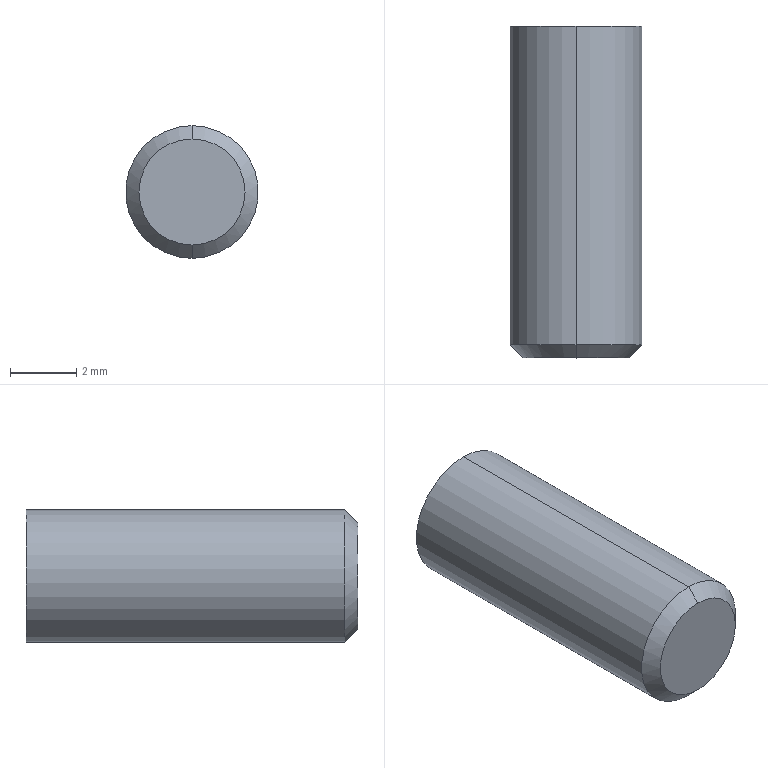Part | SolidWorks | features BaseBody 1 | 1 solid | 13 faces | box 4 x 10 x 4 mm | volume 117.243 mm3 | plane 9 | cylinder 2 | cone 2 | commonest cylinder face diameters 4 x2
STEP:
#1=CARTESIAN_POINT('',(0.,15.,10.));
#2=VERTEX_POINT('',#1);
#3=CARTESIAN_POINT('',(0.,15.,14.));
#4=VERTEX_POINT('',#3);
#5=CARTESIAN_POINT('',(0.,15.,12.));
#6=DIRECTION('',(0.,-1.,0.));
#7=DIRECTION('',(0.,0.,-1.));
#8=AXIS2_PLACEMENT_3D('',#5,#6,#7);
#9=CIRCLE('',#8,2.);
#10=EDGE_CURVE('',#2,#4,#9,.T.);
#11=ORIENTED_EDGE('',*,*,#10,.T.);
#12=CARTESIAN_POINT('',(0.,5.4,14.));
#13=VERTEX_POINT('',#12);
#14=CARTESIAN_POINT('',(0.,10.2,14.));
#15=DIRECTION('',(0.,-1.,0.));
#16=VECTOR('',#15,1000.);
#17=LINE('',#14,#16);
#18=EDGE_CURVE('',#4,#13,#17,.T.);
#19=ORIENTED_EDGE('',*,*,#18,.T.);
#20=CARTESIAN_POINT('',(0.,5.4,10.));
#21=VERTEX_POINT('',#20);
#22=CARTESIAN_POINT('',(0.,5.4,12.));
#23=DIRECTION('',(0.,1.,0.));
#24=DIRECTION('',(0.,0.,-1.));
#25=AXIS2_PLACEMENT_3D('',#22,#23,#24);
#26=CIRCLE('',#25,2.);
#27=EDGE_CURVE('',#13,#21,#26,.T.);
#28=ORIENTED_EDGE('',*,*,#27,.T.);
#29=CARTESIAN_POINT('',(0.,10.2,10.));
#30=DIRECTION('',(0.,-1.,0.));
#31=VECTOR('',#30,1000.);
#32=LINE('',#29,#31);
#33=EDGE_CURVE('',#2,#21,#32,.T.);
#34=ORIENTED_EDGE('',*,*,#33,.F.);
#35=EDGE_LOOP('',(#11,#19,#28,#34));
#36=FACE_OUTER_BOUND('',#35,.T.);
#37=CARTESIAN_POINT('',(0.,10.2,12.));
#38=DIRECTION('',(0.,-1.,0.));
#39=DIRECTION('',(0.,0.,-1.));
#40=AXIS2_PLACEMENT_3D('',#37,#38,#39);
#41=CYLINDRICAL_SURFACE('',#40,2.);
#42=ADVANCED_FACE('',(#36),#41,.T.);
#43=CARTESIAN_POINT('',(0.,5.,13.6));
#44=VERTEX_POINT('',#43);
#45=CARTESIAN_POINT('',(0.,5.,10.4));
#46=VERTEX_POINT('',#45);
#47=CARTESIAN_POINT('',(0.,5.,12.));
#48=DIRECTION('',(0.,1.,0.));
#49=DIRECTION('',(0.,0.,1.));
#50=AXIS2_PLACEMENT_3D('',#47,#48,#49);
#51=CIRCLE('',#50,1.6);
#52=EDGE_CURVE('',#44,#46,#51,.T.);
#53=ORIENTED_EDGE('',*,*,#52,.T.);
#54=CARTESIAN_POINT('',(0.,5.4,10.));
#55=DIRECTION('',(0.,0.7071,-0.7071));
#56=VECTOR('',#55,1000.);
#57=LINE('',#54,#56);
#58=EDGE_CURVE('',#46,#21,#57,.T.);
#59=ORIENTED_EDGE('',*,*,#58,.T.);
#60=ORIENTED_EDGE('',*,*,#27,.F.);
#61=CARTESIAN_POINT('',(0.,5.4,14.));
#62=DIRECTION('',(0.,0.7071,0.7071));
#63=VECTOR('',#62,1000.);
#64=LINE('',#61,#63);
#65=EDGE_CURVE('',#44,#13,#64,.T.);
#66=ORIENTED_EDGE('',*,*,#65,.F.);
#67=EDGE_LOOP('',(#53,#59,#60,#66));
#68=FACE_OUTER_BOUND('',#67,.T.);
#69=CARTESIAN_POINT('',(0.,5.4,12.));
#70=DIRECTION('',(0.,1.,0.));
#71=DIRECTION('',(0.,0.,1.));
#72=AXIS2_PLACEMENT_3D('',#69,#70,#71);
#73=CONICAL_SURFACE('',#72,2.,0.7854);
#74=ADVANCED_FACE('',(#68),#73,.T.);
#75=ORIENTED_EDGE('',*,*,#18,.F.);
#76=CARTESIAN_POINT('',(0.,15.,12.));
#77=DIRECTION('',(0.,-1.,0.));
#78=DIRECTION('',(0.,0.,-1.));
#79=AXIS2_PLACEMENT_3D('',#76,#77,#78);
#80=CIRCLE('',#79,2.);
#81=EDGE_CURVE('',#4,#2,#80,.T.);
#82=ORIENTED_EDGE('',*,*,#81,.T.);
#83=ORIENTED_EDGE('',*,*,#33,.T.);
#84=CARTESIAN_POINT('',(0.,5.4,12.));
#85=DIRECTION('',(0.,1.,0.));
#86=DIRECTION('',(0.,0.,-1.));
#87=AXIS2_PLACEMENT_3D('',#84,#85,#86);
#88=CIRCLE('',#87,2.);
#89=EDGE_CURVE('',#21,#13,#88,.T.);
#90=ORIENTED_EDGE('',*,*,#89,.T.);
#91=EDGE_LOOP('',(#75,#82,#83,#90));
#92=FACE_OUTER_BOUND('',#91,.T.);
#93=CARTESIAN_POINT('',(0.,10.2,12.));
#94=DIRECTION('',(0.,-1.,0.));
#95=DIRECTION('',(0.,0.,-1.));
#96=AXIS2_PLACEMENT_3D('',#93,#94,#95);
#97=CYLINDRICAL_SURFACE('',#96,2.);
#98=ADVANCED_FACE('',(#92),#97,.T.);
#99=ORIENTED_EDGE('',*,*,#58,.F.);
#100=CARTESIAN_POINT('',(0.,5.,12.));
#101=DIRECTION('',(0.,1.,0.));
#102=DIRECTION('',(0.,0.,1.));
#103=AXIS2_PLACEMENT_3D('',#100,#101,#102);
#104=CIRCLE('',#103,1.6);
#105=EDGE_CURVE('',#46,#44,#104,.T.);
#106=ORIENTED_EDGE('',*,*,#105,.T.);
#107=ORIENTED_EDGE('',*,*,#65,.T.);
#108=ORIENTED_EDGE('',*,*,#89,.F.);
#109=EDGE_LOOP('',(#99,#106,#107,#108));
#110=FACE_OUTER_BOUND('',#109,.T.);
#111=CARTESIAN_POINT('',(0.,5.4,12.));
#112=DIRECTION('',(0.,1.,0.));
#113=DIRECTION('',(0.,0.,1.));
#114=AXIS2_PLACEMENT_3D('',#111,#112,#113);
#115=CONICAL_SURFACE('',#114,2.,0.7854);
#116=ADVANCED_FACE('',(#110),#115,.T.);
#117=CARTESIAN_POINT('',(1.039,15.,11.4));
#118=VERTEX_POINT('',#117);
#119=CARTESIAN_POINT('',(1.039,15.,12.6));
#120=VERTEX_POINT('',#119);
#121=CARTESIAN_POINT('',(1.039,15.,12.));
#122=DIRECTION('',(0.,0.,1.));
#123=VECTOR('',#122,1000.);
#124=LINE('',#121,#123);
#125=EDGE_CURVE('',#118,#120,#124,.T.);
#126=ORIENTED_EDGE('',*,*,#125,.T.);
#127=CARTESIAN_POINT('',(0.,15.,13.2));
#128=VERTEX_POINT('',#127);
#129=CARTESIAN_POINT('',(1.039,15.,12.6));
#130=DIRECTION('',(-0.866,0.,0.5));
#131=VECTOR('',#130,1000.);
#132=LINE('',#129,#131);
#133=EDGE_CURVE('',#120,#128,#132,.T.);
#134=ORIENTED_EDGE('',*,*,#133,.T.);
#135=CARTESIAN_POINT('',(-1.039,15.,12.6));
#136=VERTEX_POINT('',#135);
#137=CARTESIAN_POINT('',(-0.5196,15.,12.9));
#138=DIRECTION('',(-0.866,0.,-0.5));
#139=VECTOR('',#138,1000.);
#140=LINE('',#137,#139);
#141=EDGE_CURVE('',#128,#136,#140,.T.);
#142=ORIENTED_EDGE('',*,*,#141,.T.);
#143=CARTESIAN_POINT('',(-1.039,15.,11.4));
#144=VERTEX_POINT('',#143);
#145=CARTESIAN_POINT('',(-1.039,15.,12.));
#146=DIRECTION('',(0.,0.,-1.));
#147=VECTOR('',#146,1000.);
#148=LINE('',#145,#147);
#149=EDGE_CURVE('',#136,#144,#148,.T.);
#150=ORIENTED_EDGE('',*,*,#149,.T.);
#151=CARTESIAN_POINT('',(0.,15.,10.8));
#152=VERTEX_POINT('',#151);
#153=CARTESIAN_POINT('',(-0.5196,15.,11.1));
#154=DIRECTION('',(0.866,0.,-0.5));
#155=VECTOR('',#154,1000.);
#156=LINE('',#153,#155);
#157=EDGE_CURVE('',#144,#152,#156,.T.);
#158=ORIENTED_EDGE('',*,*,#157,.T.);
#159=CARTESIAN_POINT('',(0.5196,15.,11.1));
#160=DIRECTION('',(0.866,0.,0.5));
#161=VECTOR('',#160,1000.);
#162=LINE('',#159,#161);
#163=EDGE_CURVE('',#152,#118,#162,.T.);
#164=ORIENTED_EDGE('',*,*,#163,.T.);
#165=EDGE_LOOP('',(#126,#134,#142,#150,#158,#164));
#166=FACE_BOUND('',#165,.T.);
#167=ORIENTED_EDGE('',*,*,#10,.F.);
#168=ORIENTED_EDGE('',*,*,#81,.F.);
#169=EDGE_LOOP('',(#167,#168));
#170=FACE_OUTER_BOUND('',#169,.T.);
#171=CARTESIAN_POINT('',(0.,15.,13.));
#172=DIRECTION('',(0.,1.,0.));
#173=DIRECTION('',(0.,0.,1.));
#174=AXIS2_PLACEMENT_3D('',#171,#172,#173);
#175=PLANE('',#174);
#176=ADVANCED_FACE('',(#166,#170),#175,.T.);
#177=ORIENTED_EDGE('',*,*,#52,.F.);
#178=ORIENTED_EDGE('',*,*,#105,.F.);
#179=EDGE_LOOP('',(#177,#178));
#180=FACE_OUTER_BOUND('',#179,.T.);
#181=CARTESIAN_POINT('',(0.,5.,12.8));
#182=DIRECTION('',(0.,-1.,0.));
#183=DIRECTION('',(0.,0.,-1.));
#184=AXIS2_PLACEMENT_3D('',#181,#182,#183);
#185=PLANE('',#184);
#186=ADVANCED_FACE('',(#180),#185,.T.);
#187=ORIENTED_EDGE('',*,*,#133,.F.);
#188=CARTESIAN_POINT('',(1.039,13.,12.6));
#189=VERTEX_POINT('',#188);
#190=CARTESIAN_POINT('',(1.039,15.,12.6));
#191=DIRECTION('',(0.,1.,0.));
#192=VECTOR('',#191,1000.);
#193=LINE('',#190,#192);
#194=EDGE_CURVE('',#189,#120,#193,.T.);
#195=ORIENTED_EDGE('',*,*,#194,.F.);
#196=CARTESIAN_POINT('',(0.,13.,13.2));
#197=VERTEX_POINT('',#196);
#198=CARTESIAN_POINT('',(0.5196,13.,12.9));
#199=DIRECTION('',(0.866,0.,-0.5));
#200=VECTOR('',#199,1000.);
#201=LINE('',#198,#200);
#202=EDGE_CURVE('',#197,#189,#201,.T.);
#203=ORIENTED_EDGE('',*,*,#202,.F.);
#204=CARTESIAN_POINT('',(0.,15.,13.2));
#205=DIRECTION('',(0.,-1.,0.));
#206=VECTOR('',#205,1000.);
#207=LINE('',#204,#206);
#208=EDGE_CURVE('',#128,#197,#207,.T.);
#209=ORIENTED_EDGE('',*,*,#208,.F.);
#210=EDGE_LOOP('',(#187,#195,#203,#209));
#211=FACE_OUTER_BOUND('',#210,.T.);
#212=CARTESIAN_POINT('',(0.5196,15.,12.9));
#213=DIRECTION('',(0.5,0.,0.866));
#214=DIRECTION('',(0.866,0.,-0.5));
#215=AXIS2_PLACEMENT_3D('',#212,#213,#214);
#216=PLANE('',#215);
#217=ADVANCED_FACE('',(#211),#216,.F.);
#218=ORIENTED_EDGE('',*,*,#141,.F.);
#219=ORIENTED_EDGE('',*,*,#208,.T.);
#220=CARTESIAN_POINT('',(-1.039,13.,12.6));
#221=VERTEX_POINT('',#220);
#222=CARTESIAN_POINT('',(-0.5196,13.,12.9));
#223=DIRECTION('',(0.866,0.,0.5));
#224=VECTOR('',#223,1000.);
#225=LINE('',#222,#224);
#226=EDGE_CURVE('',#221,#197,#225,.T.);
#227=ORIENTED_EDGE('',*,*,#226,.F.);
#228=CARTESIAN_POINT('',(-1.039,15.,12.6));
#229=DIRECTION('',(0.,-1.,0.));
#230=VECTOR('',#229,1000.);
#231=LINE('',#228,#230);
#232=EDGE_CURVE('',#136,#221,#231,.T.);
#233=ORIENTED_EDGE('',*,*,#232,.F.);
#234=EDGE_LOOP('',(#218,#219,#227,#233));
#235=FACE_OUTER_BOUND('',#234,.T.);
#236=CARTESIAN_POINT('',(-0.5196,15.,12.9));
#237=DIRECTION('',(-0.5,0.,0.866));
#238=DIRECTION('',(0.866,0.,0.5));
#239=AXIS2_PLACEMENT_3D('',#236,#237,#238);
#240=PLANE('',#239);
#241=ADVANCED_FACE('',(#235),#240,.F.);
#242=ORIENTED_EDGE('',*,*,#125,.F.);
#243=CARTESIAN_POINT('',(1.039,13.,11.4));
#244=VERTEX_POINT('',#243);
#245=CARTESIAN_POINT('',(1.039,15.,11.4));
#246=DIRECTION('',(0.,1.,0.));
#247=VECTOR('',#246,1000.);
#248=LINE('',#245,#247);
#249=EDGE_CURVE('',#244,#118,#248,.T.);
#250=ORIENTED_EDGE('',*,*,#249,.F.);
#251=CARTESIAN_POINT('',(1.039,13.,12.));
#252=DIRECTION('',(0.,0.,-1.));
#253=VECTOR('',#252,1000.);
#254=LINE('',#251,#253);
#255=EDGE_CURVE('',#189,#244,#254,.T.);
#256=ORIENTED_EDGE('',*,*,#255,.F.);
#257=ORIENTED_EDGE('',*,*,#194,.T.);
#258=EDGE_LOOP('',(#242,#250,#256,#257));
#259=FACE_OUTER_BOUND('',#258,.T.);
#260=CARTESIAN_POINT('',(1.039,15.,12.));
#261=DIRECTION('',(1.,0.,0.));
#262=DIRECTION('',(0.,0.,-1.));
#263=AXIS2_PLACEMENT_3D('',#260,#261,#262);
#264=PLANE('',#263);
#265=ADVANCED_FACE('',(#259),#264,.F.);
#266=ORIENTED_EDGE('',*,*,#226,.T.);
#267=ORIENTED_EDGE('',*,*,#202,.T.);
#268=ORIENTED_EDGE('',*,*,#255,.T.);
#269=CARTESIAN_POINT('',(0.,13.,10.8));
#270=VERTEX_POINT('',#269);
#271=CARTESIAN_POINT('',(1.039,13.,11.4));
#272=DIRECTION('',(-0.866,0.,-0.5));
#273=VECTOR('',#272,1000.);
#274=LINE('',#271,#273);
#275=EDGE_CURVE('',#244,#270,#274,.T.);
#276=ORIENTED_EDGE('',*,*,#275,.T.);
#277=CARTESIAN_POINT('',(-1.039,13.,11.4));
#278=VERTEX_POINT('',#277);
#279=CARTESIAN_POINT('',(-0.5196,13.,11.1));
#280=DIRECTION('',(-0.866,0.,0.5));
#281=VECTOR('',#280,1000.);
#282=LINE('',#279,#281);
#283=EDGE_CURVE('',#270,#278,#282,.T.);
#284=ORIENTED_EDGE('',*,*,#283,.T.);
#285=CARTESIAN_POINT('',(-1.039,13.,12.));
#286=DIRECTION('',(0.,0.,1.));
#287=VECTOR('',#286,1000.);
#288=LINE('',#285,#287);
#289=EDGE_CURVE('',#278,#221,#288,.T.);
#290=ORIENTED_EDGE('',*,*,#289,.T.);
#291=EDGE_LOOP('',(#266,#267,#268,#276,#284,#290));
#292=FACE_OUTER_BOUND('',#291,.T.);
#293=CARTESIAN_POINT('',(0.,13.,12.));
#294=DIRECTION('',(0.,1.,0.));
#295=DIRECTION('',(0.,0.,1.));
#296=AXIS2_PLACEMENT_3D('',#293,#294,#295);
#297=PLANE('',#296);
#298=ADVANCED_FACE('',(#292),#297,.T.);
#299=ORIENTED_EDGE('',*,*,#149,.F.);
#300=ORIENTED_EDGE('',*,*,#232,.T.);
#301=ORIENTED_EDGE('',*,*,#289,.F.);
#302=CARTESIAN_POINT('',(-1.039,15.,11.4));
#303=DIRECTION('',(0.,-1.,0.));
#304=VECTOR('',#303,1000.);
#305=LINE('',#302,#304);
#306=EDGE_CURVE('',#144,#278,#305,.T.);
#307=ORIENTED_EDGE('',*,*,#306,.F.);
#308=EDGE_LOOP('',(#299,#300,#301,#307));
#309=FACE_OUTER_BOUND('',#308,.T.);
#310=CARTESIAN_POINT('',(-1.039,15.,12.));
#311=DIRECTION('',(-1.,0.,0.));
#312=DIRECTION('',(0.,0.,1.));
#313=AXIS2_PLACEMENT_3D('',#310,#311,#312);
#314=PLANE('',#313);
#315=ADVANCED_FACE('',(#309),#314,.F.);
#316=ORIENTED_EDGE('',*,*,#163,.F.);
#317=CARTESIAN_POINT('',(0.,15.,10.8));
#318=DIRECTION('',(0.,1.,0.));
#319=VECTOR('',#318,1000.);
#320=LINE('',#317,#319);
#321=EDGE_CURVE('',#270,#152,#320,.T.);
#322=ORIENTED_EDGE('',*,*,#321,.F.);
#323=ORIENTED_EDGE('',*,*,#275,.F.);
#324=ORIENTED_EDGE('',*,*,#249,.T.);
#325=EDGE_LOOP('',(#316,#322,#323,#324));
#326=FACE_OUTER_BOUND('',#325,.T.);
#327=CARTESIAN_POINT('',(0.5196,15.,11.1));
#328=DIRECTION('',(0.5,0.,-0.866));
#329=DIRECTION('',(-0.866,0.,-0.5));
#330=AXIS2_PLACEMENT_3D('',#327,#328,#329);
#331=PLANE('',#330);
#332=ADVANCED_FACE('',(#326),#331,.F.);
#333=ORIENTED_EDGE('',*,*,#157,.F.);
#334=ORIENTED_EDGE('',*,*,#306,.T.);
#335=ORIENTED_EDGE('',*,*,#283,.F.);
#336=ORIENTED_EDGE('',*,*,#321,.T.);
#337=EDGE_LOOP('',(#333,#334,#335,#336));
#338=FACE_OUTER_BOUND('',#337,.T.);
#339=CARTESIAN_POINT('',(-0.5196,15.,11.1));
#340=DIRECTION('',(-0.5,0.,-0.866));
#341=DIRECTION('',(-0.866,0.,0.5));
#342=AXIS2_PLACEMENT_3D('',#339,#340,#341);
#343=PLANE('',#342);
#344=ADVANCED_FACE('',(#338),#343,.F.);
#345=CLOSED_SHELL('',(#42,#74,#98,#116,#176,#186,#217,#241,#265,#298,#315,#332,#344));
#346=MANIFOLD_SOLID_BREP('',#345);
#347=CARTESIAN_POINT('',(0.,0.,0.));
#348=DIRECTION('',(0.,0.,1.));
#349=DIRECTION('',(1.,0.,0.));
#350=AXIS2_PLACEMENT_3D('',#347,#348,#349);
#351=(LENGTH_UNIT()NAMED_UNIT(*)SI_UNIT(.MILLI.,.METRE.));
#352=UNCERTAINTY_MEASURE_WITH_UNIT(LENGTH_MEASURE(0.00001),#351,'','');
#353=(NAMED_UNIT(*)PLANE_ANGLE_UNIT()SI_UNIT($,.RADIAN.));
#354=(NAMED_UNIT(*)SI_UNIT($,.STERADIAN.)SOLID_ANGLE_UNIT());
#355=(GEOMETRIC_REPRESENTATION_CONTEXT(3)GLOBAL_UNCERTAINTY_ASSIGNED_CONTEXT((#352))GLOBAL_UNIT_ASSIGNED_CONTEXT((#351,#353,#354))REPRESENTATION_CONTEXT('',''));
#356=ADVANCED_BREP_SHAPE_REPRESENTATION('',(#346,#350),#355);